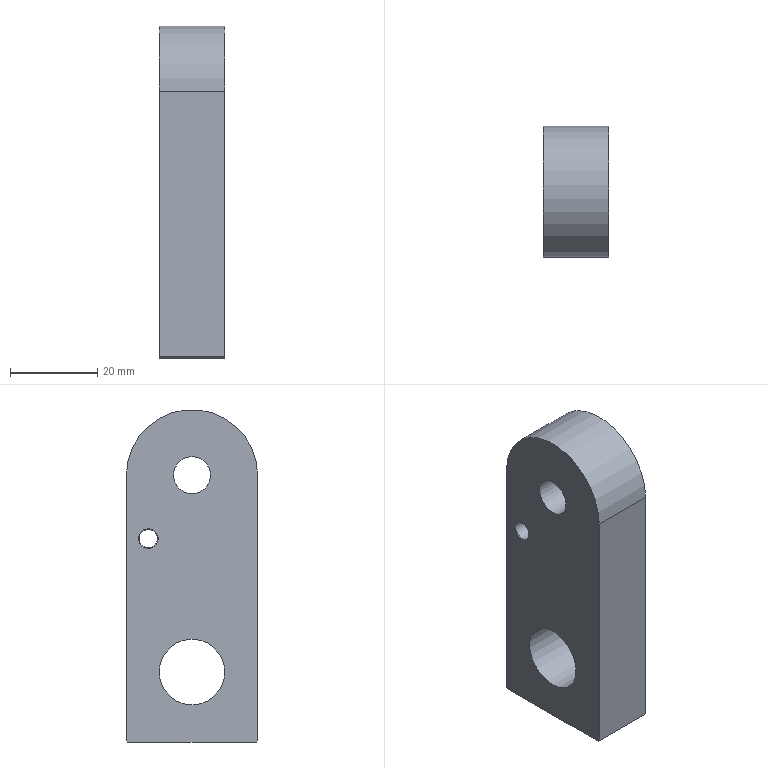NC program | NX | posted with a generic post | part box 15 x 30 x 76 mm
Lines 14123 to 14637 of 31310:
(THREAD_MILLING , TOOL : THREAD_MILL)
N28214 T16 M6
N28216 G53
N28218 G17 G0 G90 X-23. Y0. S3000 M3
N28220 G43 Z50. H16
N28222 Z-17.375
N28224 G41 G94 G3 X-22.789 Y-0.122 Z-17. I0.106 J-0.061 F150. D16
N28226 X-22.789 Y-0.122 Z-15.5 I-0.211 J0.122
N28228 X-23. Y0. Z-15.125 I-0.106 J0.061
N28230 G40
N28232 G0 Z-12.875
N28234 G41 G3 X-22.789 Y-0.122 Z-12.5 I0.106 J-0.061
N28236 X-22.789 Y-0.122 Z-11. I-0.211 J0.122
N28238 X-23. Y0. Z-10.625 I-0.106 J0.061
N28240 G40
N28242 G0 Z-8.375
N28244 G41 G3 X-22.789 Y-0.122 Z-8. I0.106 J-0.061
N28246 X-22.789 Y-0.122 Z-6.5 I-0.211 J0.122
N28248 X-23. Y0. Z-6.125 I-0.106 J0.061
N28250 G40
N28252 G0 Z-3.875
N28254 G41 G3 X-22.789 Y-0.122 Z-3.5 I0.106 J-0.061
N28256 X-22.789 Y-0.122 Z-2. I-0.211 J0.122
N28258 X-23. Y0. Z-1.625 I-0.106 J0.061
N28260 G40
N28262 G0 Z-17.375
N28264 G41 G3 X-22.708 Y-0.169 Z-17. I0.146 J-0.084
N28266 X-22.708 Y-0.169 Z-15.5 I-0.292 J0.169
N28268 X-23. Y0. Z-15.125 I-0.146 J0.084
N28270 G40
N28272 G0 Z-12.875
N28274 G41 G3 X-22.708 Y-0.169 Z-12.5 I0.146 J-0.084
N28276 X-22.708 Y-0.169 Z-11. I-0.292 J0.169
N28278 X-23. Y0. Z-10.625 I-0.146 J0.084
N28280 G40
N28282 G0 Z-8.375
N28284 G41 G3 X-22.708 Y-0.169 Z-8. I0.146 J-0.084
N28286 X-22.708 Y-0.169 Z-6.5 I-0.292 J0.169
N28288 X-23. Y0. Z-6.125 I-0.146 J0.084
N28290 G40
N28292 G0 Z-3.875
N28294 G41 G3 X-22.708 Y-0.169 Z-3.5 I0.146 J-0.084
N28296 X-22.708 Y-0.169 Z-2. I-0.292 J0.169
N28298 X-23. Y0. Z-1.625 I-0.146 J0.084
N28300 G40
N28302 G0 Z-17.375
N28304 G41 G3 X-22.627 Y-0.216 Z-17. I0.187 J-0.108
N28306 X-22.627 Y-0.216 Z-15.5 I-0.373 J0.216
N28308 X-23. Y0. Z-15.125 I-0.187 J0.108
N28310 G40
N28312 G0 Z-12.875
N28314 G41 G3 X-22.627 Y-0.216 Z-12.5 I0.187 J-0.108
N28316 X-22.627 Y-0.216 Z-11. I-0.373 J0.216
N28318 X-23. Y0. Z-10.625 I-0.187 J0.108
N28320 G40
N28322 G0 Z-8.375
N28324 G41 G3 X-22.627 Y-0.216 Z-8. I0.187 J-0.108
N28326 X-22.627 Y-0.216 Z-6.5 I-0.373 J0.216
N28328 X-23. Y0. Z-6.125 I-0.187 J0.108
N28330 G40
N28332 G0 Z-3.875
N28334 G41 G3 X-22.627 Y-0.216 Z-3.5 I0.187 J-0.108
N28336 X-22.627 Y-0.216 Z-2. I-0.373 J0.216
N28338 X-23. Y0. Z-1.625 I-0.187 J0.108
N28340 G40
N28342 G0 Z-17.019
N28344 G41 G1 X-22.582 Y-0.275
N28346 X-22.568 Y-0.28 Z-17.013
N28348 X-22.553 Y-0.275 Z-17.006
N28350 X-22.545 Y-0.263 Z-17.
N28352 G3 X-22.545 Y-0.263 Z-15.5 I-0.455 J0.263
N28354 G1 X-22.538 Y-0.249 Z-15.494
N28356 X-22.542 Y-0.234 Z-15.487
N28358 X-22.553 Y-0.224 Z-15.481
N28360 G40
N28362 X-23. Y0.
N28364 G0 Z-12.519
N28366 G41 G1 X-22.582 Y-0.275
N28368 X-22.568 Y-0.28 Z-12.513
N28370 X-22.553 Y-0.275 Z-12.506
N28372 X-22.545 Y-0.263 Z-12.5
N28374 G3 X-22.545 Y-0.263 Z-11. I-0.455 J0.262
N28376 G1 X-22.538 Y-0.249 Z-10.994
N28378 X-22.542 Y-0.234 Z-10.987
N28380 X-22.553 Y-0.224 Z-10.981
N28382 G40
N28384 X-23. Y0.
N28386 G0 Z-8.019
N28388 G41 G1 X-22.582 Y-0.275
N28390 X-22.568 Y-0.28 Z-8.013
N28392 X-22.553 Y-0.275 Z-8.006
N28394 X-22.545 Y-0.263 Z-8.
N28396 G3 X-22.545 Y-0.263 Z-6.5 I-0.455 J0.262
N28398 G1 X-22.538 Y-0.249 Z-6.494
N28400 X-22.542 Y-0.234 Z-6.487
N28402 X-22.553 Y-0.224 Z-6.481
N28404 G40
N28406 X-23. Y0.
N28408 G0 Z-3.519
N28410 G41 G1 X-22.582 Y-0.275
N28412 X-22.568 Y-0.28 Z-3.513
N28414 X-22.553 Y-0.275 Z-3.506
N28416 X-22.545 Y-0.263 Z-3.5
N28418 G3 X-22.545 Y-0.263 Z-2. I-0.455 J0.262
N28420 G1 X-22.538 Y-0.249 Z-1.994
N28422 X-22.542 Y-0.234 Z-1.987
N28424 X-22.553 Y-0.224 Z-1.981
N28426 G40
N28428 X-23. Y0.
N28430 G0 Z-17.079
N28432 G41 G1 X-22.643 Y-0.35
N28434 G3 X-22.464 Y-0.309 Z-17. R0.125
N28436 X-22.464 Y-0.309 Z-15.5 I-0.536 J0.309
N28438 X-22.518 Y-0.134 Z-15.421 R0.125
N28440 G40
N28442 G1 X-23. Y0.
N28444 G0 Z-12.579
N28446 G41 G1 X-22.643 Y-0.35
N28448 G3 X-22.464 Y-0.309 Z-12.5 R0.125
N28450 X-22.464 Y-0.309 Z-11. I-0.536 J0.309
N28452 X-22.518 Y-0.134 Z-10.921 R0.125
N28454 G40
N28456 G1 X-23. Y0.
N28458 G0 Z-8.079
N28460 G41 G1 X-22.643 Y-0.35
N28462 G3 X-22.464 Y-0.309 Z-8. R0.125
N28464 X-22.464 Y-0.309 Z-6.5 I-0.536 J0.309
N28466 X-22.518 Y-0.134 Z-6.421 R0.125
N28468 G40
N28470 G1 X-23. Y0.
N28472 G0 Z-3.579
N28474 G41 G1 X-22.643 Y-0.35
N28476 G3 X-22.464 Y-0.309 Z-3.5 R0.125
N28478 X-22.464 Y-0.309 Z-2. I-0.536 J0.309
N28480 X-22.518 Y-0.134 Z-1.921 R0.125
N28482 G40
N28484 G1 X-23. Y0.
N28486 G0 Z-17.125
N28488 G41 G1 X-22.703 Y-0.402
N28490 G3 X-22.383 Y-0.356 Z-17. R0.206
N28492 X-22.383 Y-0.356 Z-15.5 I-0.617 J0.356
N28494 X-22.503 Y-0.056 Z-15.375 R0.206
N28496 G40
N28498 G1 X-23. Y0.
N28500 G0 Z-12.625
N28502 G41 G1 X-22.703 Y-0.402
N28504 G3 X-22.383 Y-0.356 Z-12.5 R0.206
N28506 X-22.383 Y-0.356 Z-11. I-0.617 J0.356
N28508 X-22.503 Y-0.056 Z-10.875 R0.206
N28510 G40
N28512 G1 X-23. Y0.
N28514 G0 Z-8.125
N28516 G41 G1 X-22.703 Y-0.402
N28518 G3 X-22.383 Y-0.356 Z-8. R0.206
N28520 X-22.383 Y-0.356 Z-6.5 I-0.617 J0.356
N28522 X-22.503 Y-0.056 Z-6.375 R0.206
N28524 G40
N28526 G1 X-23. Y0.
N28528 G0 Z-3.625
N28530 G41 G1 X-22.703 Y-0.402
N28532 G3 X-22.383 Y-0.356 Z-3.5 R0.206
N28534 X-22.383 Y-0.356 Z-2. I-0.617 J0.356
N28536 X-22.503 Y-0.056 Z-1.875 R0.206
N28538 G40
N28540 G1 X-23. Y0.
N28542 G0 Z-17.16
N28544 G41 G1 X-22.759 Y-0.438
N28546 G3 X-22.302 Y-0.403 Z-17. R0.278
N28548 X-22.302 Y-0.403 Z-15.5 I-0.698 J0.403
N28550 X-22.5 Y0.011 Z-15.34 R0.278
N28552 G40
N28554 G1 X-23. Y0.
N28556 G0 Z-12.66
N28558 G41 G1 X-22.759 Y-0.438
N28560 G3 X-22.302 Y-0.403 Z-12.5 R0.278
N28562 X-22.302 Y-0.403 Z-11. I-0.698 J0.403
N28564 X-22.5 Y0.011 Z-10.84 R0.278
N28566 G40
N28568 G1 X-23. Y0.
N28570 G0 Z-8.16
N28572 G41 G1 X-22.759 Y-0.438
N28574 G3 X-22.302 Y-0.403 Z-8. R0.278
N28576 X-22.302 Y-0.403 Z-6.5 I-0.698 J0.403
N28578 X-22.5 Y0.011 Z-6.34 R0.278
N28580 G40
N28582 G1 X-23. Y0.
N28584 G0 Z-3.66
N28586 G41 G1 X-22.759 Y-0.438
N28588 G3 X-22.302 Y-0.403 Z-3.5 R0.278
N28590 X-22.302 Y-0.403 Z-2. I-0.698 J0.403
N28592 X-22.5 Y0.011 Z-1.84 R0.278
N28594 G40
N28596 G1 X-23. Y0.
N28598 G0 Z-17.187
N28600 G41 G1 X-22.81 Y-0.462
N28602 G3 X-22.221 Y-0.45 Z-17. R0.344
N28604 X-22.221 Y-0.45 Z-15.5 I-0.779 J0.45
N28606 X-22.504 Y0.066 Z-15.313 R0.344
N28608 G40
N28610 G1 X-23. Y0.
N28612 G0 Z-12.687
N28614 G41 G1 X-22.81 Y-0.462
N28616 G3 X-22.221 Y-0.45 Z-12.5 R0.344
N28618 X-22.221 Y-0.45 Z-11. I-0.779 J0.45
N28620 X-22.504 Y0.066 Z-10.813 R0.344
N28622 G40
N28624 G1 X-23. Y0.
N28626 G0 Z-8.187
N28628 G41 G1 X-22.81 Y-0.462
N28630 G3 X-22.221 Y-0.45 Z-8. R0.344
N28632 X-22.221 Y-0.45 Z-6.5 I-0.779 J0.45
N28634 X-22.504 Y0.066 Z-6.313 R0.344
N28636 G40
N28638 G1 X-23. Y0.
N28640 G0 Z-3.687
N28642 G41 G1 X-22.81 Y-0.462
N28644 G3 X-22.221 Y-0.45 Z-3.5 R0.344
N28646 X-22.221 Y-0.45 Z-2. I-0.779 J0.45
N28648 X-22.504 Y0.066 Z-1.813 R0.344
N28650 G40
N28652 G1 X-23. Y0.
N28654 G0 Z-17.187
N28656 G41 G1 X-22.81 Y-0.462
N28658 G3 X-22.221 Y-0.45 Z-17. R0.344
N28660 X-22.221 Y-0.45 Z-15.5 I-0.779 J0.45
N28662 X-22.504 Y0.066 Z-15.313 R0.344
N28664 G40
N28666 G1 X-23. Y0.
N28668 G0 Z-12.687
N28670 G41 G1 X-22.81 Y-0.462
N28672 G3 X-22.221 Y-0.45 Z-12.5 R0.344
N28674 X-22.221 Y-0.45 Z-11. I-0.779 J0.45
N28676 X-22.504 Y0.066 Z-10.813 R0.344
N28678 G40
N28680 G1 X-23. Y0.
N28682 G0 Z-8.187
N28684 G41 G1 X-22.81 Y-0.462
N28686 G3 X-22.221 Y-0.45 Z-8. R0.344
N28688 X-22.221 Y-0.45 Z-6.5 I-0.779 J0.45
N28690 X-22.504 Y0.066 Z-6.313 R0.344
N28692 G40
N28694 G1 X-23. Y0.
N28696 G0 Z-3.687
N28698 G41 G1 X-22.81 Y-0.462
N28700 G3 X-22.221 Y-0.45 Z-3.5 R0.344
N28702 X-22.221 Y-0.45 Z-2. I-0.779 J0.45
N28704 X-22.504 Y0.066 Z-1.813 R0.344
N28706 G40
N28708 G1 X-23. Y0.
N28710 G0 Z-17.187
N28712 G41 G1 X-22.81 Y-0.462
N28714 G3 X-22.221 Y-0.45 Z-17. R0.344
N28716 X-22.221 Y-0.45 Z-15.5 I-0.779 J0.45
N28718 X-22.504 Y0.066 Z-15.313 R0.344
N28720 G40
N28722 G1 X-23. Y0.
N28724 G0 Z-12.687
N28726 G41 G1 X-22.81 Y-0.462
N28728 G3 X-22.221 Y-0.45 Z-12.5 R0.344
N28730 X-22.221 Y-0.45 Z-11. I-0.779 J0.45
N28732 X-22.504 Y0.066 Z-10.813 R0.344
N28734 G40
N28736 G1 X-23. Y0.
N28738 G0 Z-8.187
N28740 G41 G1 X-22.81 Y-0.462
N28742 G3 X-22.221 Y-0.45 Z-8. R0.344
N28744 X-22.221 Y-0.45 Z-6.5 I-0.779 J0.45
N28746 X-22.504 Y0.066 Z-6.313 R0.344
N28748 G40
N28750 G1 X-23. Y0.
N28752 G0 Z-3.687
N28754 G41 G1 X-22.81 Y-0.462
N28756 G3 X-22.221 Y-0.45 Z-3.5 R0.344
N28758 X-22.221 Y-0.45 Z-2. I-0.779 J0.45
N28760 X-22.504 Y0.066 Z-1.813 R0.344
N28762 G40
N28764 G1 X-23. Y0.
N28766 G0 Z50.
N28768 M5
(HOLE_MILLING_COPY , TOOL : D6.)
N28770 T05 M6
N28772 G53
N28774 G17 G0 G90 X22. Y0. S2800 M3
N28776 G43 Z50. H5
N28778 Z0.5
N28780 G41 G94 G1 X22.1 Y0.004 F800. D5
N28782 G3 X22. Y4.4 R2.199
N28784 X22. Y4.4 Z0.3 I0. J-4.4
N28786 X22. Y4.4 Z0.1 I0. J-4.4
N28788 X22. Y4.4 Z-0.1 I0. J-4.4
N28790 X22. Y4.4 Z-0.3 I0. J-4.4
N28792 X22. Y4.4 Z-0.5 I0. J-4.4
N28794 X22. Y4.4 Z-0.7 I0. J-4.4
N28796 X22. Y4.4 Z-0.9 I0. J-4.4
N28798 X22. Y4.4 Z-1.1 I0. J-4.4
N28800 X22. Y4.4 Z-1.3 I0. J-4.4
N28802 X22. Y4.4 Z-1.5 I0. J-4.4
N28804 X22. Y4.4 Z-1.7 I0. J-4.4
N28806 X22. Y4.4 Z-1.9 I0. J-4.4
N28808 X22. Y4.4 Z-2.1 I0. J-4.4
N28810 X22. Y4.4 Z-2.3 I0. J-4.4
N28812 X22. Y4.4 Z-2.5 I0. J-4.4
N28814 X22. Y4.4 Z-2.7 I0. J-4.4
N28816 X22. Y4.4 Z-2.9 I0. J-4.4
N28818 X22. Y4.4 Z-3.1 I0. J-4.4
N28820 X22. Y4.4 Z-3.3 I0. J-4.4
N28822 X22. Y4.4 Z-3.5 I0. J-4.4
N28824 X22. Y4.4 Z-3.7 I0. J-4.4
N28826 X22. Y4.4 Z-3.9 I0. J-4.4
N28828 X22. Y4.4 Z-4.1 I0. J-4.4
N28830 X22. Y4.4 Z-4.3 I0. J-4.4
N28832 X22. Y4.4 Z-4.5 I0. J-4.4
N28834 X22. Y4.4 Z-4.7 I0. J-4.4
N28836 X22. Y4.4 Z-4.9 I0. J-4.4
N28838 X22. Y4.4 Z-5.1 I0. J-4.4
N28840 X22. Y4.4 Z-5.3 I0. J-4.4
N28842 X22. Y4.4 Z-5.5 I0. J-4.4
N28844 X22. Y4.4 Z-5.7 I0. J-4.4
N28846 X22. Y4.4 Z-5.9 I0. J-4.4
N28848 X22. Y4.4 Z-6.1 I0. J-4.4
N28850 X22. Y4.4 Z-6.3 I0. J-4.4
N28852 X22. Y4.4 Z-6.5 I0. J-4.4
N28854 X22. Y4.4 Z-6.7 I0. J-4.4
N28856 X22. Y4.4 Z-6.9 I0. J-4.4
N28858 X22. Y4.4 Z-7.1 I0. J-4.4
N28860 X22. Y4.4 Z-7.3 I0. J-4.4
N28862 X22. Y4.4 Z-7.5 I0. J-4.4
N28864 X22. Y4.4 Z-7.7 I0. J-4.4
N28866 X22. Y4.4 Z-7.9 I0. J-4.4
N28868 X22. Y4.4 Z-8.1 I0. J-4.4
N28870 X22. Y4.4 Z-8.3 I0. J-4.4
N28872 X22. Y4.4 Z-8.5 I0. J-4.4
N28874 X22. Y4.4 Z-8.7 I0. J-4.4
N28876 X22. Y4.4 Z-8.9 I0. J-4.4
N28878 X22. Y4.4 Z-9.1 I0. J-4.4
N28880 X22. Y4.4 Z-9.3 I0. J-4.4
N28882 X22. Y4.4 Z-9.5 I0. J-4.4
N28884 X22. Y4.4 Z-9.7 I0. J-4.4
N28886 X22. Y4.4 Z-9.9 I0. J-4.4
N28888 X22. Y4.4 Z-10.1 I0. J-4.4
N28890 X22. Y4.4 Z-10.3 I0. J-4.4
N28892 X22. Y4.4 Z-10.5 I0. J-4.4
N28894 X22. Y4.4 Z-10.7 I0. J-4.4
N28896 X22. Y4.4 Z-10.9 I0. J-4.4
N28898 X22. Y4.4 Z-11.1 I0. J-4.4
N28900 X22. Y4.4 Z-11.3 I0. J-4.4
N28902 X22. Y4.4 Z-11.5 I0. J-4.4
N28904 X22. Y4.4 Z-11.7 I0. J-4.4
N28906 X22. Y4.4 Z-11.9 I0. J-4.4
N28908 X22. Y4.4 Z-12.1 I0. J-4.4
N28910 X22. Y4.4 Z-12.3 I0. J-4.4
N28912 X22. Y4.4 Z-12.5 I0. J-4.4
N28914 X22. Y4.4 Z-12.7 I0. J-4.4
N28916 X22. Y4.4 Z-12.9 I0. J-4.4
N28918 X22. Y4.4 Z-13.1 I0. J-4.4
N28920 X22. Y4.4 Z-13.3 I0. J-4.4
N28922 X22. Y4.4 Z-13.5 I0. J-4.4
N28924 X22. Y4.4 Z-13.7 I0. J-4.4
N28926 X22. Y4.4 Z-13.9 I0. J-4.4
N28928 X22. Y4.4 Z-14.1 I0. J-4.4
N28930 X22. Y4.4 Z-14.3 I0. J-4.4
N28932 X22. Y4.4 Z-14.5 I0. J-4.4
N28934 X22. Y4.4 Z-14.7 I0. J-4.4
N28936 X22. Y4.4 Z-14.9 I0. J-4.4
N28938 X22. Y4.4 Z-15.1 I0. J-4.4
N28940 X22. Y4.4 Z-15.3 I0. J-4.4
N28942 X22. Y4.4 Z-15.5 I0. J-4.4
N28944 X22. Y4.4 Z-15.7 I0. J-4.4
N28946 X22. Y4.4 Z-15.9 I0. J-4.4
N28948 X22. Y-4.4 Z-16. I0. J-4.4
N28950 X26.4 Y0. R4.4
N28952 X22. Y-4.4 R-4.4
N28954 X22.1 Y-0.004 R2.199
N28956 G40
N28958 G1 X22. Y0.
N28960 G0 Z50.
(PLANAR_MILL_2 , TOOL : D6.)
N28962 X23.269 Y-1.965 S3000
N28964 Z-13.5
N28966 G1 Z-15.5 F300.
N28968 G41 X23.466 Y-2.
N28970 X24.48
N28972 G3 X26.48 Y0. R2.
N28974 X22. Y4.48 R4.48
N28976 X26.48 Y0. R-4.48
N28978 X24.48 Y2. R2.
N28980 G40
N28982 G1 X24.283 Y1.965
N28984 Y-1.965
N28986 G41 X24.48 Y-2.
N28988 G3 X26.48 Y0. R2.
N28990 X22. Y4.48 R4.48
N28992 X26.48 Y0. R-4.48
N28994 X24.48 Y2. R2.
N28996 G40
N28998 G1 X24.283 Y1.965
N29000 Y-1.965
N29002 G41 X24.48 Y-2.
N29004 G3 X26.48 Y0. R2.
N29006 X22. Y4.48 R4.48
N29008 X26.48 Y0. R-4.48
N29010 X24.48 Y2. R2.
N29012 G1 X23.466
N29014 G40
N29016 X23.269 Y1.965
N29018 Z-13.5
N29020 G0 Z50.
N29022 M5
(FLOOR_FACING_COPY_2_1_COPY_COPY , TOOL : D63精)
N29024 T18 M6
N29026 G53
N29028 G17 G0 G90 X-79.5 Y0. S1800 M3
N29030 G43 Z50. H18
N29032 Z3.
N29034 G94 G1 Z0. F400.
N29036 X-69.5
N29038 X69.5
N29040 X79.5
N29042 Z3.
N29044 G0 Z50.
N29046 M5
(PLANAR_MILL , TOOL : D10精光)
N29048 T02 M6
N29050 G53
N29052 G17 G0 G90 X39.68 Y-21.766 S2000 M3
N29054 G43 Z50. H2
N29056 Z-15.5
N29058 G94 G3 X37.7 Y-20.05 R2. F400.
N29060 G1 X-23.
N29062 G2 X-43.05 Y0. R20.05
N29064 X-23. Y20.05 R20.05
N29066 G1 X37.7
N29068 G2 X41.271 Y18.571 R5.05
N29070 G1 X41.571 Y18.271
N29072 G2 X43.05 Y14.7 R5.05
N29074 G1 Y-14.7
N29076 G2 X41.571 Y-18.271 R5.05
N29078 G1 X41.271 Y-18.571
N29080 G2 X37.7 Y-20.05 R5.05
N29082 G3 X35.7 Y-22.05 R2.
N29084 G1 X39.686 Y-21.764
N29086 G3 X37.7 Y-20. R2.
N29088 G1 X-23.
N29090 G2 X-43. Y0. R20.
N29092 X-23. Y20. R20.
N29094 G1 X37.7
N29096 G2 X41.236 Y18.536 R5.
N29098 G1 X41.536 Y18.236
N29100 G2 X43. Y14.7 R5.
N29102 G1 Y-14.7
N29104 G2 X41.536 Y-18.236 R5.
N29106 G1 X41.236 Y-18.536
N29108 G2 X37.7 Y-20. R5.
N29110 G3 X35.7 Y-22.05 R2.001
N29112 G0 Z50.
N29114 M5
(PLANAR_MILL_COPY , TOOL : 4倒角)
N29116 T19 M6
N29118 G53
N29120 G17 G0 G90 X-24.878 Y19.083 S5000 M3
N29122 G43 Z50. H19
N29124 Z-1.5
N29126 G41 G94 G1 X-24.997 Y18.09 F600. D19
N29128 G3 X-23. Y16.2 R2.
N29130 G1 X37.576
N29132 G2 X38.636 Y15.761 R1.5
N29134 G1 X38.761 Y15.636
N29136 G2 X39.2 Y14.576 R1.5
N29138 G1 Y-14.576
N29140 G2 X38.761 Y-15.636 R1.5
N29142 G1 X38.636 Y-15.761
N29144 G2 X37.576 Y-16.2 R1.5
N29146 G1 X-23.
N29148 G2 X-39.2 Y0. R16.2
N29150 X-23. Y16.2 R16.2
N29152 G3 X-21. Y18.2 R2.
N29154 G40
N29156 G1 X-21.174 Y19.185
N29158 G0 Z50.
(PLANAR_MILL_COPY_COPY , TOOL : 4倒角)
N29160 X19.178 Y1.826
N29162 Z-1.5
N29164 G41 G1 X18.193 Y2.
N29166 X17.7
N29168 G3 X15.7 Y0. R2.
N29170 X22. Y-6.3 R6.3
N29172 X15.7 Y0. R-6.3
N29174 X17.7 Y-2. R2.
N29176 G40
N29178 G1 X18.685 Y-1.826
N29180 Y1.826
N29182 G41 X17.7 Y2.
N29184 G3 X15.7 Y0. R2.
N29186 X22. Y-6.3 R6.3
N29188 X15.7 Y0. R-6.3
N29190 X17.7 Y-2. R2.
N29192 G1 X18.193
N29194 G40
N29196 X19.178 Y-1.826
N29198 G0 Z50.
N29200 M5